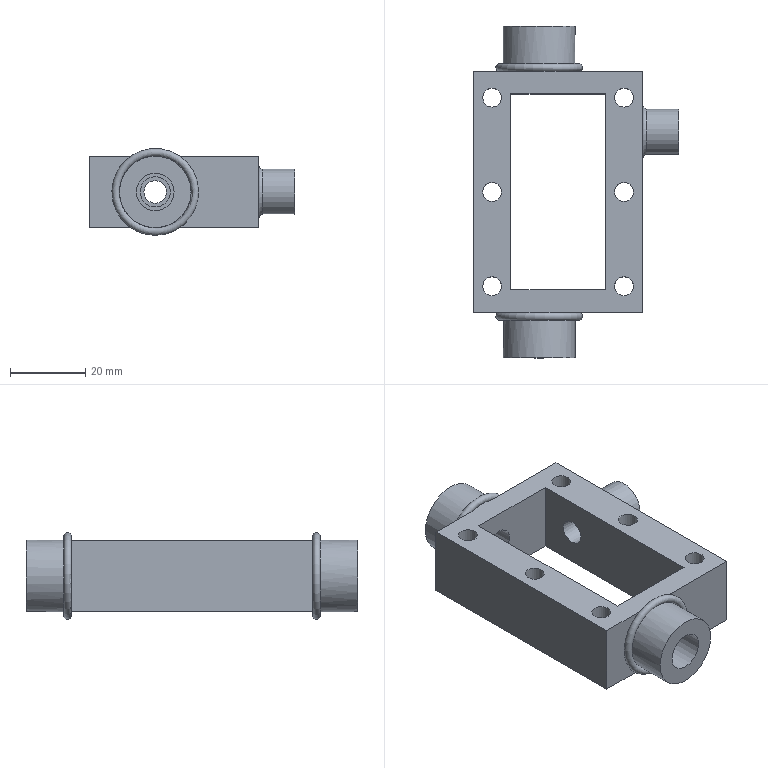Part | STEP file | 1-06.8 | 1 solid | 42 faces | box 54.5 x 88 x 23 mm | volume 33301 mm3 | plane 19 | cylinder 16 | torus 7 | commonest cylinder face diameters 5 x7 8 x2 10 x2 19 x2 6 x1 6.5 x1